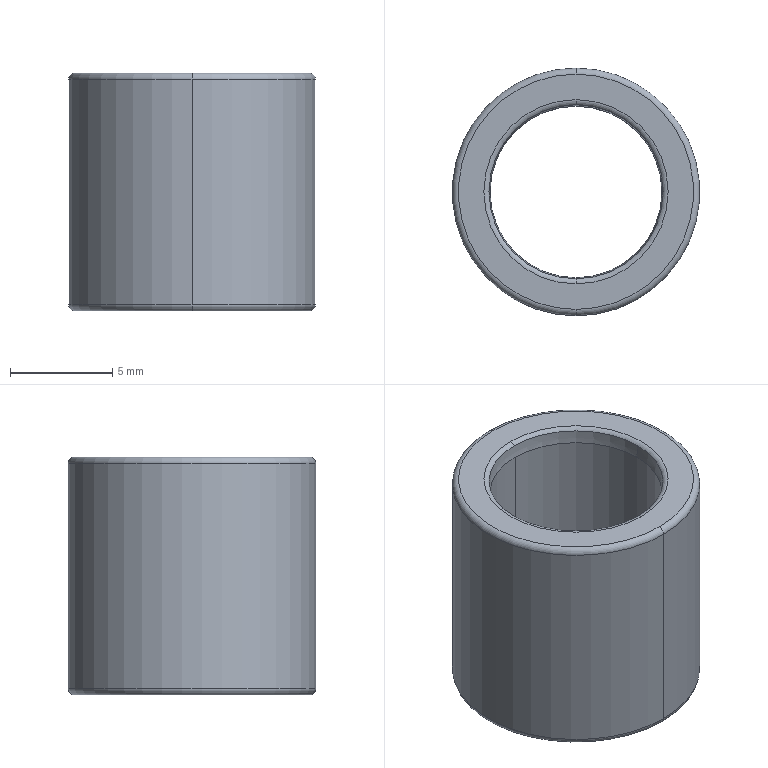Part | STEP file | 12b-1_03 | 1 solid | 16 faces | box 12.07 x 12.07 x 11.6 mm | volume 683.04 mm3 | torus 8 | cylinder 4 | plane 2 | spline 2 | commonest cylinder face diameters 8.39 x2 12.07 x2
STEP:
#1=CARTESIAN_POINT('',(0.,0.,0.));
#2=DIRECTION('',(0.,0.,1.));
#3=DIRECTION('',(1.,0.,0.));
#4=AXIS2_PLACEMENT_3D('',#1,#2,#3);
#5=CARTESIAN_POINT('',(9.525,-4.195,-5.5));
#6=VERTEX_POINT('',#5);
#7=CARTESIAN_POINT('',(9.525,-4.495,-5.8));
#8=VERTEX_POINT('',#7);
#9=CARTESIAN_POINT('',(9.525,-4.495,-5.5));
#10=DIRECTION('',(-1.,0.,0.));
#11=DIRECTION('',(0.,1.,0.));
#12=AXIS2_PLACEMENT_3D('',#9,#10,#11);
#13=CIRCLE('',#12,0.3);
#14=CARTESIAN_POINT('',(9.525,0.,-5.5));
#15=DIRECTION('',(0.,0.,1.));
#16=DIRECTION('',(-0.03665,-0.9993,0.));
#17=AXIS2_PLACEMENT_3D('',#14,#15,#16);
#18=TOROIDAL_SURFACE('',#17,4.495,0.3);
#19=CARTESIAN_POINT('',(0.03666,3.142));
#20=DIRECTION('',(0.,1.));
#21=VECTOR('',#20,1.);
#22=LINE('',#19,#21);
#23=(GEOMETRIC_REPRESENTATION_CONTEXT(2)PARAMETRIC_REPRESENTATION_CONTEXT()REPRESENTATION_CONTEXT('',''));
#24=DEFINITIONAL_REPRESENTATION('',(#22),#23);
#25=PCURVE('',#18,#24);
#26=CARTESIAN_POINT('',(9.525,0.,-5.5));
#27=DIRECTION('',(0.,0.,1.));
#28=DIRECTION('',(0.03665,0.9993,0.));
#29=AXIS2_PLACEMENT_3D('',#26,#27,#28);
#30=TOROIDAL_SURFACE('',#29,4.495,0.3);
#31=CARTESIAN_POINT('',(3.178,3.142));
#32=DIRECTION('',(0.,1.));
#33=VECTOR('',#32,1.);
#34=LINE('',#31,#33);
#35=(GEOMETRIC_REPRESENTATION_CONTEXT(2)PARAMETRIC_REPRESENTATION_CONTEXT()REPRESENTATION_CONTEXT('',''));
#36=DEFINITIONAL_REPRESENTATION('',(#34),#35);
#37=PCURVE('',#30,#36);
#38=SURFACE_CURVE('',#13,(#25,#37),.PCURVE_S1.);
#39=EDGE_CURVE('',#6,#8,#38,.T.);
#40=ORIENTED_EDGE('',*,*,#39,.F.);
#41=CARTESIAN_POINT('',(9.525,4.195,-5.5));
#42=VERTEX_POINT('',#41);
#43=CARTESIAN_POINT('',(9.525,0.,-5.5));
#44=DIRECTION('',(0.,0.,-1.));
#45=DIRECTION('',(0.,1.,0.));
#46=AXIS2_PLACEMENT_3D('',#43,#44,#45);
#47=CIRCLE('',#46,4.195);
#48=CARTESIAN_POINT('',(3.178,3.142));
#49=DIRECTION('',(-1.,0.));
#50=VECTOR('',#49,1.);
#51=LINE('',#48,#50);
#52=(GEOMETRIC_REPRESENTATION_CONTEXT(2)PARAMETRIC_REPRESENTATION_CONTEXT()REPRESENTATION_CONTEXT('',''));
#53=DEFINITIONAL_REPRESENTATION('',(#51),#52);
#54=PCURVE('',#18,#53);
#55=CARTESIAN_POINT('',(9.525,0.,-5.5));
#56=DIRECTION('',(0.,0.,-1.));
#57=DIRECTION('',(0.,1.,0.));
#58=AXIS2_PLACEMENT_3D('',#55,#56,#57);
#59=CYLINDRICAL_SURFACE('',#58,4.195);
#60=CARTESIAN_POINT('',(0.,0.));
#61=DIRECTION('',(1.,0.));
#62=VECTOR('',#61,1.);
#63=LINE('',#60,#62);
#64=(GEOMETRIC_REPRESENTATION_CONTEXT(2)PARAMETRIC_REPRESENTATION_CONTEXT()REPRESENTATION_CONTEXT('',''));
#65=DEFINITIONAL_REPRESENTATION('',(#63),#64);
#66=PCURVE('',#59,#65);
#67=SURFACE_CURVE('',#47,(#54,#66),.PCURVE_S1.);
#68=EDGE_CURVE('',#42,#6,#67,.T.);
#69=ORIENTED_EDGE('',*,*,#68,.F.);
#70=CARTESIAN_POINT('',(9.525,4.495,-5.8));
#71=VERTEX_POINT('',#70);
#72=CARTESIAN_POINT('',(9.525,4.495,-5.5));
#73=DIRECTION('',(-1.,0.,0.));
#74=DIRECTION('',(0.,-0.000000819,-1.));
#75=AXIS2_PLACEMENT_3D('',#72,#73,#74);
#76=CIRCLE('',#75,0.3);
#77=CARTESIAN_POINT('',(3.178,4.712));
#78=DIRECTION('',(0.,-1.));
#79=VECTOR('',#78,1.);
#80=LINE('',#77,#79);
#81=(GEOMETRIC_REPRESENTATION_CONTEXT(2)PARAMETRIC_REPRESENTATION_CONTEXT()REPRESENTATION_CONTEXT('',''));
#82=DEFINITIONAL_REPRESENTATION('',(#80),#81);
#83=PCURVE('',#18,#82);
#84=CARTESIAN_POINT('',(0.03666,4.712));
#85=DIRECTION('',(0.,-1.));
#86=VECTOR('',#85,1.);
#87=LINE('',#84,#86);
#88=(GEOMETRIC_REPRESENTATION_CONTEXT(2)PARAMETRIC_REPRESENTATION_CONTEXT()REPRESENTATION_CONTEXT('',''));
#89=DEFINITIONAL_REPRESENTATION('',(#87),#88);
#90=PCURVE('',#30,#89);
#91=SURFACE_CURVE('',#76,(#83,#90),.PCURVE_S1.);
#92=EDGE_CURVE('',#71,#42,#91,.T.);
#93=ORIENTED_EDGE('',*,*,#92,.F.);
#94=CARTESIAN_POINT('',(9.525,0.,-5.8));
#95=DIRECTION('',(0.,0.,-1.));
#96=DIRECTION('',(0.,1.,0.));
#97=AXIS2_PLACEMENT_3D('',#94,#95,#96);
#98=CIRCLE('',#97,4.495);
#99=CARTESIAN_POINT('',(3.178,4.712));
#100=DIRECTION('',(-1.,0.));
#101=VECTOR('',#100,1.);
#102=LINE('',#99,#101);
#103=(GEOMETRIC_REPRESENTATION_CONTEXT(2)PARAMETRIC_REPRESENTATION_CONTEXT()REPRESENTATION_CONTEXT('',''));
#104=DEFINITIONAL_REPRESENTATION('',(#102),#103);
#105=PCURVE('',#18,#104);
#106=CARTESIAN_POINT('',(9.525,0.,-5.8));
#107=DIRECTION('',(0.,0.,1.));
#108=DIRECTION('',(1.,0.,0.));
#109=AXIS2_PLACEMENT_3D('',#106,#107,#108);
#110=PLANE('',#109);
#111=CARTESIAN_POINT('',(0.,4.495));
#112=CARTESIAN_POINT('',(7.786,4.495));
#113=CARTESIAN_POINT('',(3.893,-2.247));
#114=CARTESIAN_POINT('',(0.,-8.99));
#115=CARTESIAN_POINT('',(-3.893,-2.247));
#116=CARTESIAN_POINT('',(-7.786,4.495));
#117=CARTESIAN_POINT('',(0.,4.495));
#118=(BOUNDED_CURVE()B_SPLINE_CURVE(2,(#111,#112,#113,#114,#115,#116,#117),.UNSPECIFIED.,.T.,.F.)B_SPLINE_CURVE_WITH_KNOTS((1,2,2,2,2,1),(-2.094,0.,2.094,4.189,6.283,8.378),.UNSPECIFIED.)CURVE()GEOMETRIC_REPRESENTATION_ITEM()RATIONAL_B_SPLINE_CURVE((1.,0.5,1.,0.5,1.,0.5,1.))REPRESENTATION_ITEM(''));
#119=(GEOMETRIC_REPRESENTATION_CONTEXT(2)PARAMETRIC_REPRESENTATION_CONTEXT()REPRESENTATION_CONTEXT('',''));
#120=DEFINITIONAL_REPRESENTATION('',(#118),#119);
#121=PCURVE('',#110,#120);
#122=SURFACE_CURVE('',#98,(#105,#121),.PCURVE_S1.);
#123=EDGE_CURVE('',#71,#8,#122,.T.);
#124=ORIENTED_EDGE('',*,*,#123,.T.);
#125=EDGE_LOOP('',(#40,#69,#93,#124));
#126=FACE_BOUND('',#125,.T.);
#127=ADVANCED_FACE('',(#126),#18,.T.);
#128=CARTESIAN_POINT('',(9.525,-5.735,-5.8));
#129=VERTEX_POINT('',#128);
#130=CARTESIAN_POINT('',(9.525,5.735,-5.8));
#131=VERTEX_POINT('',#130);
#132=CARTESIAN_POINT('',(9.525,0.,-5.8));
#133=DIRECTION('',(0.,0.,1.));
#134=DIRECTION('',(0.,-1.,0.));
#135=AXIS2_PLACEMENT_3D('',#132,#133,#134);
#136=CIRCLE('',#135,5.735);
#137=CARTESIAN_POINT('',(0.,0.));
#138=DIRECTION('',(0.,-1.));
#139=AXIS2_PLACEMENT_2D('',#137,#138);
#140=CIRCLE('',#139,5.735);
#141=(GEOMETRIC_REPRESENTATION_CONTEXT(2)PARAMETRIC_REPRESENTATION_CONTEXT()REPRESENTATION_CONTEXT('',''));
#142=DEFINITIONAL_REPRESENTATION('',(#140),#141);
#143=PCURVE('',#110,#142);
#144=CARTESIAN_POINT('',(9.525,0.,-5.5));
#145=DIRECTION('',(0.,0.,1.));
#146=DIRECTION('',(-0.03619,0.9993,0.));
#147=AXIS2_PLACEMENT_3D('',#144,#145,#146);
#148=TOROIDAL_SURFACE('',#147,5.735,0.3);
#149=CARTESIAN_POINT('',(3.105,4.712));
#150=DIRECTION('',(1.,0.));
#151=VECTOR('',#150,1.);
#152=LINE('',#149,#151);
#153=(GEOMETRIC_REPRESENTATION_CONTEXT(2)PARAMETRIC_REPRESENTATION_CONTEXT()REPRESENTATION_CONTEXT('',''));
#154=DEFINITIONAL_REPRESENTATION('',(#152),#153);
#155=PCURVE('',#148,#154);
#156=SURFACE_CURVE('',#136,(#143,#155),.PCURVE_S1.);
#157=EDGE_CURVE('',#129,#131,#156,.T.);
#158=ORIENTED_EDGE('',*,*,#157,.F.);
#159=CARTESIAN_POINT('',(9.525,0.,-5.8));
#160=DIRECTION('',(0.,0.,1.));
#161=DIRECTION('',(0.,1.,0.));
#162=AXIS2_PLACEMENT_3D('',#159,#160,#161);
#163=CIRCLE('',#162,5.735);
#164=CARTESIAN_POINT('',(0.,0.));
#165=DIRECTION('',(0.,1.));
#166=AXIS2_PLACEMENT_2D('',#164,#165);
#167=CIRCLE('',#166,5.735);
#168=(GEOMETRIC_REPRESENTATION_CONTEXT(2)PARAMETRIC_REPRESENTATION_CONTEXT()REPRESENTATION_CONTEXT('',''));
#169=DEFINITIONAL_REPRESENTATION('',(#167),#168);
#170=PCURVE('',#110,#169);
#171=CARTESIAN_POINT('',(9.525,0.,-5.5));
#172=DIRECTION('',(0.,0.,1.));
#173=DIRECTION('',(0.03619,-0.9993,0.));
#174=AXIS2_PLACEMENT_3D('',#171,#172,#173);
#175=TOROIDAL_SURFACE('',#174,5.735,0.3);
#176=CARTESIAN_POINT('',(3.105,4.712));
#177=DIRECTION('',(1.,0.));
#178=VECTOR('',#177,1.);
#179=LINE('',#176,#178);
#180=(GEOMETRIC_REPRESENTATION_CONTEXT(2)PARAMETRIC_REPRESENTATION_CONTEXT()REPRESENTATION_CONTEXT('',''));
#181=DEFINITIONAL_REPRESENTATION('',(#179),#180);
#182=PCURVE('',#175,#181);
#183=SURFACE_CURVE('',#163,(#170,#182),.PCURVE_S1.);
#184=EDGE_CURVE('',#131,#129,#183,.T.);
#185=ORIENTED_EDGE('',*,*,#184,.F.);
#186=EDGE_LOOP('',(#158,#185));
#187=FACE_BOUND('',#186,.T.);
#188=CARTESIAN_POINT('',(9.525,0.,-5.8));
#189=DIRECTION('',(0.,0.,-1.));
#190=DIRECTION('',(0.,-1.,0.));
#191=AXIS2_PLACEMENT_3D('',#188,#189,#190);
#192=CIRCLE('',#191,4.495);
#193=CARTESIAN_POINT('',(0.,-4.495));
#194=CARTESIAN_POINT('',(-7.786,-4.495));
#195=CARTESIAN_POINT('',(-3.893,2.247));
#196=CARTESIAN_POINT('',(0.,8.99));
#197=CARTESIAN_POINT('',(3.893,2.247));
#198=CARTESIAN_POINT('',(7.786,-4.495));
#199=CARTESIAN_POINT('',(0.,-4.495));
#200=(BOUNDED_CURVE()B_SPLINE_CURVE(2,(#193,#194,#195,#196,#197,#198,#199),.UNSPECIFIED.,.T.,.F.)B_SPLINE_CURVE_WITH_KNOTS((1,2,2,2,2,1),(-2.094,0.,2.094,4.189,6.283,8.378),.UNSPECIFIED.)CURVE()GEOMETRIC_REPRESENTATION_ITEM()RATIONAL_B_SPLINE_CURVE((1.,0.5,1.,0.5,1.,0.5,1.))REPRESENTATION_ITEM(''));
#201=(GEOMETRIC_REPRESENTATION_CONTEXT(2)PARAMETRIC_REPRESENTATION_CONTEXT()REPRESENTATION_CONTEXT('',''));
#202=DEFINITIONAL_REPRESENTATION('',(#200),#201);
#203=PCURVE('',#110,#202);
#204=CARTESIAN_POINT('',(3.178,4.712));
#205=DIRECTION('',(-1.,0.));
#206=VECTOR('',#205,1.);
#207=LINE('',#204,#206);
#208=(GEOMETRIC_REPRESENTATION_CONTEXT(2)PARAMETRIC_REPRESENTATION_CONTEXT()REPRESENTATION_CONTEXT('',''));
#209=DEFINITIONAL_REPRESENTATION('',(#207),#208);
#210=PCURVE('',#30,#209);
#211=SURFACE_CURVE('',#192,(#203,#210),.PCURVE_S1.);
#212=EDGE_CURVE('',#8,#71,#211,.T.);
#213=ORIENTED_EDGE('',*,*,#212,.F.);
#214=ORIENTED_EDGE('',*,*,#123,.F.);
#215=EDGE_LOOP('',(#213,#214));
#216=FACE_BOUND('',#215,.T.);
#217=ADVANCED_FACE('',(#187,#216),#110,.F.);
#218=CARTESIAN_POINT('',(9.525,-6.035,-5.5));
#219=VERTEX_POINT('',#218);
#220=CARTESIAN_POINT('',(9.525,-5.735,-5.5));
#221=DIRECTION('',(-1.,0.,0.));
#222=DIRECTION('',(0.,0.000001786,-1.));
#223=AXIS2_PLACEMENT_3D('',#220,#221,#222);
#224=CIRCLE('',#223,0.3);
#225=CARTESIAN_POINT('',(6.247,4.712));
#226=DIRECTION('',(0.,1.));
#227=VECTOR('',#226,1.);
#228=LINE('',#225,#227);
#229=(GEOMETRIC_REPRESENTATION_CONTEXT(2)PARAMETRIC_REPRESENTATION_CONTEXT()REPRESENTATION_CONTEXT('',''));
#230=DEFINITIONAL_REPRESENTATION('',(#228),#229);
#231=PCURVE('',#175,#230);
#232=CARTESIAN_POINT('',(3.105,4.712));
#233=DIRECTION('',(0.,1.));
#234=VECTOR('',#233,1.);
#235=LINE('',#232,#234);
#236=(GEOMETRIC_REPRESENTATION_CONTEXT(2)PARAMETRIC_REPRESENTATION_CONTEXT()REPRESENTATION_CONTEXT('',''));
#237=DEFINITIONAL_REPRESENTATION('',(#235),#236);
#238=PCURVE('',#148,#237);
#239=SURFACE_CURVE('',#224,(#231,#238),.PCURVE_S1.);
#240=EDGE_CURVE('',#129,#219,#239,.T.);
#241=ORIENTED_EDGE('',*,*,#240,.T.);
#242=CARTESIAN_POINT('',(9.525,6.035,-5.5));
#243=VERTEX_POINT('',#242);
#244=CARTESIAN_POINT('',(9.525,0.,-5.5));
#245=DIRECTION('',(0.,0.,-1.));
#246=DIRECTION('',(0.000000001,-1.,0.));
#247=AXIS2_PLACEMENT_3D('',#244,#245,#246);
#248=CIRCLE('',#247,6.035);
#249=CARTESIAN_POINT('',(6.247,6.283));
#250=DIRECTION('',(-1.,0.));
#251=VECTOR('',#250,1.);
#252=LINE('',#249,#251);
#253=(GEOMETRIC_REPRESENTATION_CONTEXT(2)PARAMETRIC_REPRESENTATION_CONTEXT()REPRESENTATION_CONTEXT('',''));
#254=DEFINITIONAL_REPRESENTATION('',(#252),#253);
#255=PCURVE('',#175,#254);
#256=CARTESIAN_POINT('',(9.525,0.,-5.5));
#257=DIRECTION('',(0.,0.,-1.));
#258=DIRECTION('',(0.,1.,0.));
#259=AXIS2_PLACEMENT_3D('',#256,#257,#258);
#260=CYLINDRICAL_SURFACE('',#259,6.035);
#261=CARTESIAN_POINT('',(3.142,0.));
#262=DIRECTION('',(1.,0.));
#263=VECTOR('',#262,1.);
#264=LINE('',#261,#263);
#265=(GEOMETRIC_REPRESENTATION_CONTEXT(2)PARAMETRIC_REPRESENTATION_CONTEXT()REPRESENTATION_CONTEXT('',''));
#266=DEFINITIONAL_REPRESENTATION('',(#264),#265);
#267=PCURVE('',#260,#266);
#268=SURFACE_CURVE('',#248,(#255,#267),.PCURVE_S1.);
#269=EDGE_CURVE('',#219,#243,#268,.T.);
#270=ORIENTED_EDGE('',*,*,#269,.T.);
#271=CARTESIAN_POINT('',(9.525,5.735,-5.5));
#272=DIRECTION('',(-1.,0.,0.));
#273=DIRECTION('',(0.,1.,0.));
#274=AXIS2_PLACEMENT_3D('',#271,#272,#273);
#275=CIRCLE('',#274,0.3);
#276=CARTESIAN_POINT('',(3.105,6.283));
#277=DIRECTION('',(0.,-1.));
#278=VECTOR('',#277,1.);
#279=LINE('',#276,#278);
#280=(GEOMETRIC_REPRESENTATION_CONTEXT(2)PARAMETRIC_REPRESENTATION_CONTEXT()REPRESENTATION_CONTEXT('',''));
#281=DEFINITIONAL_REPRESENTATION('',(#279),#280);
#282=PCURVE('',#175,#281);
#283=CARTESIAN_POINT('',(6.247,6.283));
#284=DIRECTION('',(0.,-1.));
#285=VECTOR('',#284,1.);
#286=LINE('',#283,#285);
#287=(GEOMETRIC_REPRESENTATION_CONTEXT(2)PARAMETRIC_REPRESENTATION_CONTEXT()REPRESENTATION_CONTEXT('',''));
#288=DEFINITIONAL_REPRESENTATION('',(#286),#287);
#289=PCURVE('',#148,#288);
#290=SURFACE_CURVE('',#275,(#282,#289),.PCURVE_S1.);
#291=EDGE_CURVE('',#243,#131,#290,.T.);
#292=ORIENTED_EDGE('',*,*,#291,.T.);
#293=ORIENTED_EDGE('',*,*,#184,.T.);
#294=EDGE_LOOP('',(#241,#270,#292,#293));
#295=FACE_BOUND('',#294,.T.);
#296=ADVANCED_FACE('',(#295),#175,.T.);
#297=ORIENTED_EDGE('',*,*,#291,.F.);
#298=CARTESIAN_POINT('',(9.525,0.,-5.5));
#299=DIRECTION('',(0.,0.,-1.));
#300=DIRECTION('',(0.,1.,0.));
#301=AXIS2_PLACEMENT_3D('',#298,#299,#300);
#302=CIRCLE('',#301,6.035);
#303=CARTESIAN_POINT('',(6.247,6.283));
#304=DIRECTION('',(-1.,0.));
#305=VECTOR('',#304,1.);
#306=LINE('',#303,#305);
#307=(GEOMETRIC_REPRESENTATION_CONTEXT(2)PARAMETRIC_REPRESENTATION_CONTEXT()REPRESENTATION_CONTEXT('',''));
#308=DEFINITIONAL_REPRESENTATION('',(#306),#307);
#309=PCURVE('',#148,#308);
#310=CARTESIAN_POINT('',(9.525,0.,-5.5));
#311=DIRECTION('',(0.,0.,-1.));
#312=DIRECTION('',(0.,1.,0.));
#313=AXIS2_PLACEMENT_3D('',#310,#311,#312);
#314=CYLINDRICAL_SURFACE('',#313,6.035);
#315=CARTESIAN_POINT('',(0.,0.));
#316=DIRECTION('',(1.,0.));
#317=VECTOR('',#316,1.);
#318=LINE('',#315,#317);
#319=(GEOMETRIC_REPRESENTATION_CONTEXT(2)PARAMETRIC_REPRESENTATION_CONTEXT()REPRESENTATION_CONTEXT('',''));
#320=DEFINITIONAL_REPRESENTATION('',(#318),#319);
#321=PCURVE('',#314,#320);
#322=SURFACE_CURVE('',#302,(#309,#321),.PCURVE_S1.);
#323=EDGE_CURVE('',#243,#219,#322,.T.);
#324=ORIENTED_EDGE('',*,*,#323,.T.);
#325=ORIENTED_EDGE('',*,*,#240,.F.);
#326=ORIENTED_EDGE('',*,*,#157,.T.);
#327=EDGE_LOOP('',(#297,#324,#325,#326));
#328=FACE_BOUND('',#327,.T.);
#329=ADVANCED_FACE('',(#328),#148,.T.);
#330=CARTESIAN_POINT('',(9.525,-6.035,5.5));
#331=VERTEX_POINT('',#330);
#332=CARTESIAN_POINT('',(9.525,-6.035,5.5));
#333=DIRECTION('',(0.,0.,-1.));
#334=VECTOR('',#333,1.);
#335=LINE('',#332,#334);
#336=CARTESIAN_POINT('',(3.142,-11.));
#337=DIRECTION('',(0.,1.));
#338=VECTOR('',#337,1.);
#339=LINE('',#336,#338);
#340=(GEOMETRIC_REPRESENTATION_CONTEXT(2)PARAMETRIC_REPRESENTATION_CONTEXT()REPRESENTATION_CONTEXT('',''));
#341=DEFINITIONAL_REPRESENTATION('',(#339),#340);
#342=PCURVE('',#314,#341);
#343=CARTESIAN_POINT('',(3.142,-11.));
#344=DIRECTION('',(0.,1.));
#345=VECTOR('',#344,1.);
#346=LINE('',#343,#345);
#347=(GEOMETRIC_REPRESENTATION_CONTEXT(2)PARAMETRIC_REPRESENTATION_CONTEXT()REPRESENTATION_CONTEXT('',''));
#348=DEFINITIONAL_REPRESENTATION('',(#346),#347);
#349=PCURVE('',#260,#348);
#350=SURFACE_CURVE('',#335,(#342,#349),.PCURVE_S1.);
#351=EDGE_CURVE('',#331,#219,#350,.T.);
#352=ORIENTED_EDGE('',*,*,#351,.T.);
#353=ORIENTED_EDGE('',*,*,#323,.F.);
#354=CARTESIAN_POINT('',(9.525,6.035,5.5));
#355=VERTEX_POINT('',#354);
#356=CARTESIAN_POINT('',(9.525,6.035,-5.5));
#357=DIRECTION('',(0.,0.,1.));
#358=VECTOR('',#357,1.);
#359=LINE('',#356,#358);
#360=CARTESIAN_POINT('',(0.,0.));
#361=DIRECTION('',(0.,-1.));
#362=VECTOR('',#361,1.);
#363=LINE('',#360,#362);
#364=(GEOMETRIC_REPRESENTATION_CONTEXT(2)PARAMETRIC_REPRESENTATION_CONTEXT()REPRESENTATION_CONTEXT('',''));
#365=DEFINITIONAL_REPRESENTATION('',(#363),#364);
#366=PCURVE('',#314,#365);
#367=CARTESIAN_POINT('',(6.283,0.));
#368=DIRECTION('',(0.,-1.));
#369=VECTOR('',#368,1.);
#370=LINE('',#367,#369);
#371=(GEOMETRIC_REPRESENTATION_CONTEXT(2)PARAMETRIC_REPRESENTATION_CONTEXT()REPRESENTATION_CONTEXT('',''));
#372=DEFINITIONAL_REPRESENTATION('',(#370),#371);
#373=PCURVE('',#260,#372);
#374=SURFACE_CURVE('',#359,(#366,#373),.PCURVE_S1.);
#375=EDGE_CURVE('',#243,#355,#374,.T.);
#376=ORIENTED_EDGE('',*,*,#375,.T.);
#377=CARTESIAN_POINT('',(9.525,0.,5.5));
#378=DIRECTION('',(0.,0.,-1.));
#379=DIRECTION('',(0.,1.,0.));
#380=AXIS2_PLACEMENT_3D('',#377,#378,#379);
#381=CIRCLE('',#380,6.035);
#382=CARTESIAN_POINT('',(0.,-11.));
#383=DIRECTION('',(1.,0.));
#384=VECTOR('',#383,1.);
#385=LINE('',#382,#384);
#386=(GEOMETRIC_REPRESENTATION_CONTEXT(2)PARAMETRIC_REPRESENTATION_CONTEXT()REPRESENTATION_CONTEXT('',''));
#387=DEFINITIONAL_REPRESENTATION('',(#385),#386);
#388=PCURVE('',#314,#387);
#389=CARTESIAN_POINT('',(9.525,0.,5.5));
#390=DIRECTION('',(0.,0.,1.));
#391=DIRECTION('',(-0.02548,-0.9997,0.));
#392=AXIS2_PLACEMENT_3D('',#389,#390,#391);
#393=TOROIDAL_SURFACE('',#392,5.735,0.3);
#394=CARTESIAN_POINT('',(3.167,0.));
#395=DIRECTION('',(-1.,0.));
#396=VECTOR('',#395,1.);
#397=LINE('',#394,#396);
#398=(GEOMETRIC_REPRESENTATION_CONTEXT(2)PARAMETRIC_REPRESENTATION_CONTEXT()REPRESENTATION_CONTEXT('',''));
#399=DEFINITIONAL_REPRESENTATION('',(#397),#398);
#400=PCURVE('',#393,#399);
#401=SURFACE_CURVE('',#381,(#388,#400),.PCURVE_S1.);
#402=EDGE_CURVE('',#355,#331,#401,.T.);
#403=ORIENTED_EDGE('',*,*,#402,.T.);
#404=EDGE_LOOP('',(#352,#353,#376,#403));
#405=FACE_BOUND('',#404,.T.);
#406=ADVANCED_FACE('',(#405),#314,.T.);
#407=CARTESIAN_POINT('',(9.525,-5.735,5.8));
#408=VERTEX_POINT('',#407);
#409=CARTESIAN_POINT('',(9.525,-5.735,5.5));
#410=DIRECTION('',(1.,0.,0.));
#411=DIRECTION('',(0.,0.000001986,1.));
#412=AXIS2_PLACEMENT_3D('',#409,#410,#411);
#413=CIRCLE('',#412,0.3);
#414=CARTESIAN_POINT('',(0.02548,1.571));
#415=DIRECTION('',(0.,-1.));
#416=VECTOR('',#415,1.);
#417=LINE('',#414,#416);
#418=(GEOMETRIC_REPRESENTATION_CONTEXT(2)PARAMETRIC_REPRESENTATION_CONTEXT()REPRESENTATION_CONTEXT('',''));
#419=DEFINITIONAL_REPRESENTATION('',(#417),#418);
#420=PCURVE('',#393,#419);
#421=CARTESIAN_POINT('',(9.525,0.,5.5));
#422=DIRECTION('',(0.,0.,1.));
#423=DIRECTION('',(0.02548,0.9997,0.));
#424=AXIS2_PLACEMENT_3D('',#421,#422,#423);
#425=TOROIDAL_SURFACE('',#424,5.735,0.3);
#426=CARTESIAN_POINT('',(3.167,1.571));
#427=DIRECTION('',(0.,-1.));
#428=VECTOR('',#427,1.);
#429=LINE('',#426,#428);
#430=(GEOMETRIC_REPRESENTATION_CONTEXT(2)PARAMETRIC_REPRESENTATION_CONTEXT()REPRESENTATION_CONTEXT('',''));
#431=DEFINITIONAL_REPRESENTATION('',(#429),#430);
#432=PCURVE('',#425,#431);
#433=SURFACE_CURVE('',#413,(#420,#432),.PCURVE_S1.);
#434=EDGE_CURVE('',#408,#331,#433,.T.);
#435=ORIENTED_EDGE('',*,*,#434,.T.);
#436=ORIENTED_EDGE('',*,*,#402,.F.);
#437=CARTESIAN_POINT('',(9.525,5.735,5.8));
#438=VERTEX_POINT('',#437);
#439=CARTESIAN_POINT('',(9.525,5.735,5.5));
#440=DIRECTION('',(1.,0.,0.));
#441=DIRECTION('',(0.,1.,0.));
#442=AXIS2_PLACEMENT_3D('',#439,#440,#441);
#443=CIRCLE('',#442,0.3);
#444=CARTESIAN_POINT('',(3.167,0.));
#445=DIRECTION('',(0.,1.));
#446=VECTOR('',#445,1.);
#447=LINE('',#444,#446);
#448=(GEOMETRIC_REPRESENTATION_CONTEXT(2)PARAMETRIC_REPRESENTATION_CONTEXT()REPRESENTATION_CONTEXT('',''));
#449=DEFINITIONAL_REPRESENTATION('',(#447),#448);
#450=PCURVE('',#393,#449);
#451=CARTESIAN_POINT('',(0.02548,0.));
#452=DIRECTION('',(0.,1.));
#453=VECTOR('',#452,1.);
#454=LINE('',#451,#453);
#455=(GEOMETRIC_REPRESENTATION_CONTEXT(2)PARAMETRIC_REPRESENTATION_CONTEXT()REPRESENTATION_CONTEXT('',''));
#456=DEFINITIONAL_REPRESENTATION('',(#454),#455);
#457=PCURVE('',#425,#456);
#458=SURFACE_CURVE('',#443,(#450,#457),.PCURVE_S1.);
#459=EDGE_CURVE('',#355,#438,#458,.T.);
#460=ORIENTED_EDGE('',*,*,#459,.T.);
#461=CARTESIAN_POINT('',(9.525,0.,5.8));
#462=DIRECTION('',(0.,0.,-1.));
#463=DIRECTION('',(0.,1.,0.));
#464=AXIS2_PLACEMENT_3D('',#461,#462,#463);
#465=CIRCLE('',#464,5.735);
#466=CARTESIAN_POINT('',(3.167,1.571));
#467=DIRECTION('',(-1.,0.));
#468=VECTOR('',#467,1.);
#469=LINE('',#466,#468);
#470=(GEOMETRIC_REPRESENTATION_CONTEXT(2)PARAMETRIC_REPRESENTATION_CONTEXT()REPRESENTATION_CONTEXT('',''));
#471=DEFINITIONAL_REPRESENTATION('',(#469),#470);
#472=PCURVE('',#393,#471);
#473=CARTESIAN_POINT('',(9.525,0.,5.8));
#474=DIRECTION('',(0.,0.,1.));
#475=DIRECTION('',(1.,0.,0.));
#476=AXIS2_PLACEMENT_3D('',#473,#474,#475);
#477=PLANE('',#476);
#478=CARTESIAN_POINT('',(0.,5.735));
#479=CARTESIAN_POINT('',(9.933,5.735));
#480=CARTESIAN_POINT('',(4.967,-2.867));
#481=CARTESIAN_POINT('',(0.,-11.47));
#482=CARTESIAN_POINT('',(-4.967,-2.867));
#483=CARTESIAN_POINT('',(-9.933,5.735));
#484=CARTESIAN_POINT('',(0.,5.735));
#485=(BOUNDED_CURVE()B_SPLINE_CURVE(2,(#478,#479,#480,#481,#482,#483,#484),.UNSPECIFIED.,.T.,.F.)B_SPLINE_CURVE_WITH_KNOTS((1,2,2,2,2,1),(-2.094,0.,2.094,4.189,6.283,8.378),.UNSPECIFIED.)CURVE()GEOMETRIC_REPRESENTATION_ITEM()RATIONAL_B_SPLINE_CURVE((1.,0.5,1.,0.5,1.,0.5,1.))REPRESENTATION_ITEM(''));
#486=(GEOMETRIC_REPRESENTATION_CONTEXT(2)PARAMETRIC_REPRESENTATION_CONTEXT()REPRESENTATION_CONTEXT('',''));
#487=DEFINITIONAL_REPRESENTATION('',(#485),#486);
#488=PCURVE('',#477,#487);
#489=SURFACE_CURVE('',#465,(#472,#488),.PCURVE_S1.);
#490=EDGE_CURVE('',#438,#408,#489,.T.);
#491=ORIENTED_EDGE('',*,*,#490,.T.);
#492=EDGE_LOOP('',(#435,#436,#460,#491));
#493=FACE_BOUND('',#492,.T.);
#494=ADVANCED_FACE('',(#493),#393,.T.);
#495=ORIENTED_EDGE('',*,*,#490,.F.);
#496=CARTESIAN_POINT('',(9.525,0.,5.8));
#497=DIRECTION('',(0.,0.,-1.));
#498=DIRECTION('',(0.,-1.,0.));
#499=AXIS2_PLACEMENT_3D('',#496,#497,#498);
#500=CIRCLE('',#499,5.735);
#501=CARTESIAN_POINT('',(0.,-5.735));
#502=CARTESIAN_POINT('',(-9.933,-5.735));
#503=CARTESIAN_POINT('',(-4.967,2.867));
#504=CARTESIAN_POINT('',(0.,11.47));
#505=CARTESIAN_POINT('',(4.967,2.867));
#506=CARTESIAN_POINT('',(9.933,-5.735));
#507=CARTESIAN_POINT('',(0.,-5.735));
#508=(BOUNDED_CURVE()B_SPLINE_CURVE(2,(#501,#502,#503,#504,#505,#506,#507),.UNSPECIFIED.,.T.,.F.)B_SPLINE_CURVE_WITH_KNOTS((1,2,2,2,2,1),(-2.094,0.,2.094,4.189,6.283,8.378),.UNSPECIFIED.)CURVE()GEOMETRIC_REPRESENTATION_ITEM()RATIONAL_B_SPLINE_CURVE((1.,0.5,1.,0.5,1.,0.5,1.))REPRESENTATION_ITEM(''));
#509=(GEOMETRIC_REPRESENTATION_CONTEXT(2)PARAMETRIC_REPRESENTATION_CONTEXT()REPRESENTATION_CONTEXT('',''));
#510=DEFINITIONAL_REPRESENTATION('',(#508),#509);
#511=PCURVE('',#477,#510);
#512=CARTESIAN_POINT('',(3.167,1.571));
#513=DIRECTION('',(-1.,0.));
#514=VECTOR('',#513,1.);
#515=LINE('',#512,#514);
#516=(GEOMETRIC_REPRESENTATION_CONTEXT(2)PARAMETRIC_REPRESENTATION_CONTEXT()REPRESENTATION_CONTEXT('',''));
#517=DEFINITIONAL_REPRESENTATION('',(#515),#516);
#518=PCURVE('',#425,#517);
#519=SURFACE_CURVE('',#500,(#511,#518),.PCURVE_S1.);
#520=EDGE_CURVE('',#408,#438,#519,.T.);
#521=ORIENTED_EDGE('',*,*,#520,.F.);
#522=EDGE_LOOP('',(#495,#521));
#523=FACE_BOUND('',#522,.T.);
#524=CARTESIAN_POINT('',(9.525,4.495,5.8));
#525=VERTEX_POINT('',#524);
#526=CARTESIAN_POINT('',(9.525,-4.495,5.8));
#527=VERTEX_POINT('',#526);
#528=CARTESIAN_POINT('',(9.525,0.,5.8));
#529=DIRECTION('',(0.,0.,1.));
#530=DIRECTION('',(0.,1.,0.));
#531=AXIS2_PLACEMENT_3D('',#528,#529,#530);
#532=CIRCLE('',#531,4.495);
#533=CARTESIAN_POINT('',(0.,0.));
#534=DIRECTION('',(0.,1.));
#535=AXIS2_PLACEMENT_2D('',#533,#534);
#536=CIRCLE('',#535,4.495);
#537=(GEOMETRIC_REPRESENTATION_CONTEXT(2)PARAMETRIC_REPRESENTATION_CONTEXT()REPRESENTATION_CONTEXT('',''));
#538=DEFINITIONAL_REPRESENTATION('',(#536),#537);
#539=PCURVE('',#477,#538);
#540=CARTESIAN_POINT('',(9.525,0.,5.5));
#541=DIRECTION('',(0.,0.,1.));
#542=DIRECTION('',(0.05205,-0.9986,0.));
#543=AXIS2_PLACEMENT_3D('',#540,#541,#542);
#544=TOROIDAL_SURFACE('',#543,4.495,0.3);
#545=CARTESIAN_POINT('',(3.09,1.571));
#546=DIRECTION('',(1.,0.));
#547=VECTOR('',#546,1.);
#548=LINE('',#545,#547);
#549=(GEOMETRIC_REPRESENTATION_CONTEXT(2)PARAMETRIC_REPRESENTATION_CONTEXT()REPRESENTATION_CONTEXT('',''));
#550=DEFINITIONAL_REPRESENTATION('',(#548),#549);
#551=PCURVE('',#544,#550);
#552=SURFACE_CURVE('',#532,(#539,#551),.PCURVE_S1.);
#553=EDGE_CURVE('',#525,#527,#552,.T.);
#554=ORIENTED_EDGE('',*,*,#553,.F.);
#555=CARTESIAN_POINT('',(9.525,0.,5.8));
#556=DIRECTION('',(0.,0.,1.));
#557=DIRECTION('',(0.,-1.,0.));
#558=AXIS2_PLACEMENT_3D('',#555,#556,#557);
#559=CIRCLE('',#558,4.495);
#560=CARTESIAN_POINT('',(0.,0.));
#561=DIRECTION('',(0.,-1.));
#562=AXIS2_PLACEMENT_2D('',#560,#561);
#563=CIRCLE('',#562,4.495);
#564=(GEOMETRIC_REPRESENTATION_CONTEXT(2)PARAMETRIC_REPRESENTATION_CONTEXT()REPRESENTATION_CONTEXT('',''));
#565=DEFINITIONAL_REPRESENTATION('',(#563),#564);
#566=PCURVE('',#477,#565);
#567=CARTESIAN_POINT('',(9.525,0.,5.5));
#568=DIRECTION('',(0.,0.,1.));
#569=DIRECTION('',(-0.05205,0.9986,0.));
#570=AXIS2_PLACEMENT_3D('',#567,#568,#569);
#571=TOROIDAL_SURFACE('',#570,4.495,0.3);
#572=CARTESIAN_POINT('',(3.09,1.571));
#573=DIRECTION('',(1.,0.));
#574=VECTOR('',#573,1.);
#575=LINE('',#572,#574);
#576=(GEOMETRIC_REPRESENTATION_CONTEXT(2)PARAMETRIC_REPRESENTATION_CONTEXT()REPRESENTATION_CONTEXT('',''));
#577=DEFINITIONAL_REPRESENTATION('',(#575),#576);
#578=PCURVE('',#571,#577);
#579=SURFACE_CURVE('',#559,(#566,#578),.PCURVE_S1.);
#580=EDGE_CURVE('',#527,#525,#579,.T.);
#581=ORIENTED_EDGE('',*,*,#580,.F.);
#582=EDGE_LOOP('',(#554,#581));
#583=FACE_BOUND('',#582,.T.);
#584=ADVANCED_FACE('',(#523,#583),#477,.T.);
#585=ORIENTED_EDGE('',*,*,#459,.F.);
#586=CARTESIAN_POINT('',(9.525,0.,5.5));
#587=DIRECTION('',(0.,0.,1.));
#588=DIRECTION('',(0.,1.,0.));
#589=AXIS2_PLACEMENT_3D('',#586,#587,#588);
#590=CIRCLE('',#589,6.035);
#591=CARTESIAN_POINT('',(0.02548,0.));
#592=DIRECTION('',(1.,0.));
#593=VECTOR('',#592,1.);
#594=LINE('',#591,#593);
#595=(GEOMETRIC_REPRESENTATION_CONTEXT(2)PARAMETRIC_REPRESENTATION_CONTEXT()REPRESENTATION_CONTEXT('',''));
#596=DEFINITIONAL_REPRESENTATION('',(#594),#595);
#597=PCURVE('',#425,#596);
#598=CARTESIAN_POINT('',(6.283,-11.));
#599=DIRECTION('',(-1.,0.));
#600=VECTOR('',#599,1.);
#601=LINE('',#598,#600);
#602=(GEOMETRIC_REPRESENTATION_CONTEXT(2)PARAMETRIC_REPRESENTATION_CONTEXT()REPRESENTATION_CONTEXT('',''));
#603=DEFINITIONAL_REPRESENTATION('',(#601),#602);
#604=PCURVE('',#260,#603);
#605=SURFACE_CURVE('',#590,(#597,#604),.PCURVE_S1.);
#606=EDGE_CURVE('',#355,#331,#605,.T.);
#607=ORIENTED_EDGE('',*,*,#606,.T.);
#608=ORIENTED_EDGE('',*,*,#434,.F.);
#609=ORIENTED_EDGE('',*,*,#520,.T.);
#610=EDGE_LOOP('',(#585,#607,#608,#609));
#611=FACE_BOUND('',#610,.T.);
#612=ADVANCED_FACE('',(#611),#425,.T.);
#613=ORIENTED_EDGE('',*,*,#375,.F.);
#614=ORIENTED_EDGE('',*,*,#269,.F.);
#615=ORIENTED_EDGE('',*,*,#351,.F.);
#616=ORIENTED_EDGE('',*,*,#606,.F.);
#617=EDGE_LOOP('',(#613,#614,#615,#616));
#618=FACE_BOUND('',#617,.T.);
#619=ADVANCED_FACE('',(#618),#260,.T.);
#620=CARTESIAN_POINT('',(13.77,0.,5.666));
#621=VERTEX_POINT('',#620);
#622=CARTESIAN_POINT('',(9.525,-4.245,5.666));
#623=VERTEX_POINT('',#622);
#624=CARTESIAN_POINT('',(9.525,0.,5.666));
#625=DIRECTION('',(0.,0.,-1.));
#626=DIRECTION('',(1.,0.,0.));
#627=AXIS2_PLACEMENT_3D('',#624,#625,#626);
#628=CIRCLE('',#627,4.245);
#629=CARTESIAN_POINT('',(4.66,2.556));
#630=DIRECTION('',(-1.,0.));
#631=VECTOR('',#630,1.);
#632=LINE('',#629,#631);
#633=(GEOMETRIC_REPRESENTATION_CONTEXT(2)PARAMETRIC_REPRESENTATION_CONTEXT()REPRESENTATION_CONTEXT('',''));
#634=DEFINITIONAL_REPRESENTATION('',(#632),#633);
#635=PCURVE('',#571,#634);
#636=CARTESIAN_POINT('',(5.28,0.,5.666));
#637=CARTESIAN_POINT('',(5.28,-4.245,5.666));
#638=CARTESIAN_POINT('',(9.525,-4.245,5.666));
#639=CARTESIAN_POINT('',(13.77,-4.245,5.666));
#640=CARTESIAN_POINT('',(13.77,0.,5.666));
#641=CARTESIAN_POINT('',(5.284,0.,5.636));
#642=CARTESIAN_POINT('',(5.284,-4.241,5.636));
#643=CARTESIAN_POINT('',(9.525,-4.241,5.636));
#644=CARTESIAN_POINT('',(13.766,-4.241,5.636));
#645=CARTESIAN_POINT('',(13.766,0.,5.636));
#646=CARTESIAN_POINT('',(5.297,0.,5.5));
#647=CARTESIAN_POINT('',(5.297,-4.228,5.5));
#648=CARTESIAN_POINT('',(9.525,-4.228,5.5));
#649=CARTESIAN_POINT('',(13.753,-4.228,5.5));
#650=CARTESIAN_POINT('',(13.753,0.,5.5));
#651=CARTESIAN_POINT('',(5.297,0.,5.277));
#652=CARTESIAN_POINT('',(5.297,-4.228,5.277));
#653=CARTESIAN_POINT('',(9.525,-4.228,5.277));
#654=CARTESIAN_POINT('',(13.753,-4.228,5.277));
#655=CARTESIAN_POINT('',(13.753,0.,5.277));
#656=CARTESIAN_POINT('',(5.313,0.,5.085));
#657=CARTESIAN_POINT('',(5.313,-4.212,5.085));
#658=CARTESIAN_POINT('',(9.525,-4.212,5.085));
#659=CARTESIAN_POINT('',(13.737,-4.212,5.085));
#660=CARTESIAN_POINT('',(13.737,0.,5.085));
#661=CARTESIAN_POINT('',(5.33,0.,5.));
#662=CARTESIAN_POINT('',(5.33,-4.195,5.));
#663=CARTESIAN_POINT('',(9.525,-4.195,5.));
#664=CARTESIAN_POINT('',(13.72,-4.195,5.));
#665=CARTESIAN_POINT('',(13.72,0.,5.));
#666=(BOUNDED_SURFACE()B_SPLINE_SURFACE(3,2,((#636,#637,#638,#639,#640),(#641,#642,#643,#644,#645),(#646,#647,#648,#649,#650),(#651,#652,#653,#654,#655),(#656,#657,#658,#659,#660),(#661,#662,#663,#664,#665)),.UNSPECIFIED.,.F.,.F.,.F.)B_SPLINE_SURFACE_WITH_KNOTS((4,1,1,4),(3,2,3),(0.,0.1351,0.6114,1.),(0.,1.571,3.142),.UNSPECIFIED.)GEOMETRIC_REPRESENTATION_ITEM()RATIONAL_B_SPLINE_SURFACE(((1.,0.7071,1.,0.7071,1.),(1.,0.7071,1.,0.7071,1.),(1.,0.7071,1.,0.7071,1.),(1.,0.7071,1.,0.7071,1.),(1.,0.7071,1.,0.7071,1.),(1.,0.7071,1.,0.7071,1.)))REPRESENTATION_ITEM('')SURFACE());
#667=CARTESIAN_POINT('',(0.,3.142));
#668=CARTESIAN_POINT('',(0.,3.115));
#669=CARTESIAN_POINT('',(0.,3.063));
#670=CARTESIAN_POINT('',(0.,2.987));
#671=CARTESIAN_POINT('',(0.,2.913));
#672=CARTESIAN_POINT('',(0.,2.84));
#673=CARTESIAN_POINT('',(0.,2.768));
#674=CARTESIAN_POINT('',(0.,2.698));
#675=CARTESIAN_POINT('',(0.,2.629));
#676=CARTESIAN_POINT('',(0.,2.56));
#677=CARTESIAN_POINT('',(0.,2.492));
#678=CARTESIAN_POINT('',(0.,2.424));
#679=CARTESIAN_POINT('',(0.,2.356));
#680=CARTESIAN_POINT('',(0.,2.289));
#681=CARTESIAN_POINT('',(0.,2.221));
#682=CARTESIAN_POINT('',(0.,2.152));
#683=CARTESIAN_POINT('',(0.,2.084));
#684=CARTESIAN_POINT('',(0.,2.014));
#685=CARTESIAN_POINT('',(0.,1.944));
#686=CARTESIAN_POINT('',(0.,1.872));
#687=CARTESIAN_POINT('',(0.,1.8));
#688=CARTESIAN_POINT('',(0.,1.725));
#689=CARTESIAN_POINT('',(0.,1.649));
#690=CARTESIAN_POINT('',(0.,1.597));
#691=CARTESIAN_POINT('',(0.,1.571));
#692=B_SPLINE_CURVE_WITH_KNOTS('',3,(#667,#668,#669,#670,#671,#672,#673,#674,#675,#676,#677,#678,#679,#680,#681,#682,#683,#684,#685,#686,#687,#688,#689,#690,#691),.UNSPECIFIED.,.F.,.F.,(4,1,1,1,1,1,1,1,1,1,1,1,1,1,1,1,1,1,1,1,1,1,4),(0.,0.0714,0.1428,0.2142,0.2856,0.357,0.4284,0.4998,0.5712,0.6426,0.714,0.7854,0.8568,0.9282,0.9996,1.071,1.142,1.214,1.285,1.357,1.428,1.499,1.571),.QUASI_UNIFORM_KNOTS.);
#693=(GEOMETRIC_REPRESENTATION_CONTEXT(2)PARAMETRIC_REPRESENTATION_CONTEXT()REPRESENTATION_CONTEXT('',''));
#694=DEFINITIONAL_REPRESENTATION('',(#692),#693);
#695=PCURVE('',#666,#694);
#696=SURFACE_CURVE('',#628,(#635,#695),.PCURVE_S1.);
#697=EDGE_CURVE('',#621,#623,#696,.T.);
#698=ORIENTED_EDGE('',*,*,#697,.T.);
#699=CARTESIAN_POINT('',(9.525,-4.495,5.5));
#700=DIRECTION('',(1.,0.,0.));
#701=DIRECTION('',(0.,0.8333,0.5528));
#702=AXIS2_PLACEMENT_3D('',#699,#700,#701);
#703=CIRCLE('',#702,0.3);
#704=CARTESIAN_POINT('',(3.09,2.556));
#705=DIRECTION('',(0.,-1.));
#706=VECTOR('',#705,1.);
#707=LINE('',#704,#706);
#708=(GEOMETRIC_REPRESENTATION_CONTEXT(2)PARAMETRIC_REPRESENTATION_CONTEXT()REPRESENTATION_CONTEXT('',''));
#709=DEFINITIONAL_REPRESENTATION('',(#707),#708);
#710=PCURVE('',#571,#709);
#711=CARTESIAN_POINT('',(6.231,2.556));
#712=DIRECTION('',(0.,-1.));
#713=VECTOR('',#712,1.);
#714=LINE('',#711,#713);
#715=(GEOMETRIC_REPRESENTATION_CONTEXT(2)PARAMETRIC_REPRESENTATION_CONTEXT()REPRESENTATION_CONTEXT('',''));
#716=DEFINITIONAL_REPRESENTATION('',(#714),#715);
#717=PCURVE('',#544,#716);
#718=SURFACE_CURVE('',#703,(#710,#717),.PCURVE_S1.);
#719=EDGE_CURVE('',#623,#527,#718,.T.);
#720=ORIENTED_EDGE('',*,*,#719,.T.);
#721=ORIENTED_EDGE('',*,*,#580,.T.);
#722=CARTESIAN_POINT('',(9.525,4.245,5.666));
#723=VERTEX_POINT('',#722);
#724=CARTESIAN_POINT('',(9.525,4.495,5.5));
#725=DIRECTION('',(1.,0.,0.));
#726=DIRECTION('',(0.,-0.000000814,1.));
#727=AXIS2_PLACEMENT_3D('',#724,#725,#726);
#728=CIRCLE('',#727,0.3);
#729=CARTESIAN_POINT('',(6.231,1.571));
#730=DIRECTION('',(0.,1.));
#731=VECTOR('',#730,1.);
#732=LINE('',#729,#731);
#733=(GEOMETRIC_REPRESENTATION_CONTEXT(2)PARAMETRIC_REPRESENTATION_CONTEXT()REPRESENTATION_CONTEXT('',''));
#734=DEFINITIONAL_REPRESENTATION('',(#732),#733);
#735=PCURVE('',#571,#734);
#736=CARTESIAN_POINT('',(3.09,1.571));
#737=DIRECTION('',(0.,1.));
#738=VECTOR('',#737,1.);
#739=LINE('',#736,#738);
#740=(GEOMETRIC_REPRESENTATION_CONTEXT(2)PARAMETRIC_REPRESENTATION_CONTEXT()REPRESENTATION_CONTEXT('',''));
#741=DEFINITIONAL_REPRESENTATION('',(#739),#740);
#742=PCURVE('',#544,#741);
#743=SURFACE_CURVE('',#728,(#735,#742),.PCURVE_S1.);
#744=EDGE_CURVE('',#525,#723,#743,.T.);
#745=ORIENTED_EDGE('',*,*,#744,.T.);
#746=CARTESIAN_POINT('',(9.525,0.,5.666));
#747=DIRECTION('',(0.,0.,-1.));
#748=DIRECTION('',(0.,1.,0.));
#749=AXIS2_PLACEMENT_3D('',#746,#747,#748);
#750=CIRCLE('',#749,4.245);
#751=CARTESIAN_POINT('',(6.231,2.556));
#752=DIRECTION('',(-1.,0.));
#753=VECTOR('',#752,1.);
#754=LINE('',#751,#753);
#755=(GEOMETRIC_REPRESENTATION_CONTEXT(2)PARAMETRIC_REPRESENTATION_CONTEXT()REPRESENTATION_CONTEXT('',''));
#756=DEFINITIONAL_REPRESENTATION('',(#754),#755);
#757=PCURVE('',#571,#756);
#758=CARTESIAN_POINT('',(13.77,0.,5.666));
#759=CARTESIAN_POINT('',(13.77,4.245,5.666));
#760=CARTESIAN_POINT('',(9.525,4.245,5.666));
#761=CARTESIAN_POINT('',(5.28,4.245,5.666));
#762=CARTESIAN_POINT('',(5.28,0.,5.666));
#763=CARTESIAN_POINT('',(13.766,0.,5.636));
#764=CARTESIAN_POINT('',(13.766,4.241,5.636));
#765=CARTESIAN_POINT('',(9.525,4.241,5.636));
#766=CARTESIAN_POINT('',(5.284,4.241,5.636));
#767=CARTESIAN_POINT('',(5.284,0.,5.636));
#768=CARTESIAN_POINT('',(13.753,0.,5.5));
#769=CARTESIAN_POINT('',(13.753,4.228,5.5));
#770=CARTESIAN_POINT('',(9.525,4.228,5.5));
#771=CARTESIAN_POINT('',(5.297,4.228,5.5));
#772=CARTESIAN_POINT('',(5.297,0.,5.5));
#773=CARTESIAN_POINT('',(13.753,0.,5.277));
#774=CARTESIAN_POINT('',(13.753,4.228,5.277));
#775=CARTESIAN_POINT('',(9.525,4.228,5.277));
#776=CARTESIAN_POINT('',(5.297,4.228,5.277));
#777=CARTESIAN_POINT('',(5.297,0.,5.277));
#778=CARTESIAN_POINT('',(13.737,0.,5.085));
#779=CARTESIAN_POINT('',(13.737,4.212,5.085));
#780=CARTESIAN_POINT('',(9.525,4.212,5.085));
#781=CARTESIAN_POINT('',(5.313,4.212,5.085));
#782=CARTESIAN_POINT('',(5.313,0.,5.085));
#783=CARTESIAN_POINT('',(13.72,0.,5.));
#784=CARTESIAN_POINT('',(13.72,4.195,5.));
#785=CARTESIAN_POINT('',(9.525,4.195,5.));
#786=CARTESIAN_POINT('',(5.33,4.195,5.));
#787=CARTESIAN_POINT('',(5.33,0.,5.));
#788=(BOUNDED_SURFACE()B_SPLINE_SURFACE(3,2,((#758,#759,#760,#761,#762),(#763,#764,#765,#766,#767),(#768,#769,#770,#771,#772),(#773,#774,#775,#776,#777),(#778,#779,#780,#781,#782),(#783,#784,#785,#786,#787)),.UNSPECIFIED.,.F.,.F.,.F.)B_SPLINE_SURFACE_WITH_KNOTS((4,1,1,4),(3,2,3),(0.,0.1351,0.6114,1.),(3.142,4.712,6.283),.UNSPECIFIED.)GEOMETRIC_REPRESENTATION_ITEM()RATIONAL_B_SPLINE_SURFACE(((1.,0.7071,1.,0.7071,1.),(1.,0.7071,1.,0.7071,1.),(1.,0.7071,1.,0.7071,1.),(1.,0.7071,1.,0.7071,1.),(1.,0.7071,1.,0.7071,1.),(1.,0.7071,1.,0.7071,1.)))REPRESENTATION_ITEM('')SURFACE());
#789=CARTESIAN_POINT('',(0.,4.712));
#790=CARTESIAN_POINT('',(0.,4.686));
#791=CARTESIAN_POINT('',(0.,4.634));
#792=CARTESIAN_POINT('',(0.,4.558));
#793=CARTESIAN_POINT('',(0.,4.483));
#794=CARTESIAN_POINT('',(0.,4.411));
#795=CARTESIAN_POINT('',(0.,4.339));
#796=CARTESIAN_POINT('',(0.,4.269));
#797=CARTESIAN_POINT('',(0.,4.199));
#798=CARTESIAN_POINT('',(0.,4.131));
#799=CARTESIAN_POINT('',(0.,4.063));
#800=CARTESIAN_POINT('',(0.,3.995));
#801=CARTESIAN_POINT('',(0.,3.927));
#802=CARTESIAN_POINT('',(0.,3.859));
#803=CARTESIAN_POINT('',(0.,3.791));
#804=CARTESIAN_POINT('',(0.,3.723));
#805=CARTESIAN_POINT('',(0.,3.654));
#806=CARTESIAN_POINT('',(0.,3.585));
#807=CARTESIAN_POINT('',(0.,3.515));
#808=CARTESIAN_POINT('',(0.,3.443));
#809=CARTESIAN_POINT('',(0.,3.37));
#810=CARTESIAN_POINT('',(0.,3.296));
#811=CARTESIAN_POINT('',(0.,3.22));
#812=CARTESIAN_POINT('',(0.,3.168));
#813=CARTESIAN_POINT('',(0.,3.142));
#814=B_SPLINE_CURVE_WITH_KNOTS('',3,(#789,#790,#791,#792,#793,#794,#795,#796,#797,#798,#799,#800,#801,#802,#803,#804,#805,#806,#807,#808,#809,#810,#811,#812,#813),.UNSPECIFIED.,.F.,.F.,(4,1,1,1,1,1,1,1,1,1,1,1,1,1,1,1,1,1,1,1,1,1,4),(0.,0.0714,0.1428,0.2142,0.2856,0.357,0.4284,0.4998,0.5712,0.6426,0.714,0.7854,0.8568,0.9282,0.9996,1.071,1.142,1.214,1.285,1.357,1.428,1.499,1.571),.QUASI_UNIFORM_KNOTS.);
#815=(GEOMETRIC_REPRESENTATION_CONTEXT(2)PARAMETRIC_REPRESENTATION_CONTEXT()REPRESENTATION_CONTEXT('',''));
#816=DEFINITIONAL_REPRESENTATION('',(#814),#815);
#817=PCURVE('',#788,#816);
#818=SURFACE_CURVE('',#750,(#757,#817),.PCURVE_S1.);
#819=EDGE_CURVE('',#723,#621,#818,.T.);
#820=ORIENTED_EDGE('',*,*,#819,.T.);
#821=EDGE_LOOP('',(#698,#720,#721,#745,#820));
#822=FACE_BOUND('',#821,.T.);
#823=ADVANCED_FACE('',(#822),#571,.T.);
#824=CARTESIAN_POINT('',(9.525,4.195,5.));
#825=VERTEX_POINT('',#824);
#826=CARTESIAN_POINT('',(13.72,0.,5.));
#827=VERTEX_POINT('',#826);
#828=CARTESIAN_POINT('',(9.525,0.,5.));
#829=DIRECTION('',(0.,0.,-1.));
#830=DIRECTION('',(0.,1.,0.));
#831=AXIS2_PLACEMENT_3D('',#828,#829,#830);
#832=CIRCLE('',#831,4.195);
#833=CARTESIAN_POINT('',(1.,4.712));
#834=CARTESIAN_POINT('',(1.,4.686));
#835=CARTESIAN_POINT('',(1.,4.634));
#836=CARTESIAN_POINT('',(1.,4.558));
#837=CARTESIAN_POINT('',(1.,4.483));
#838=CARTESIAN_POINT('',(1.,4.411));
#839=CARTESIAN_POINT('',(1.,4.339));
#840=CARTESIAN_POINT('',(1.,4.269));
#841=CARTESIAN_POINT('',(1.,4.199));
#842=CARTESIAN_POINT('',(1.,4.131));
#843=CARTESIAN_POINT('',(1.,4.063));
#844=CARTESIAN_POINT('',(1.,3.995));
#845=CARTESIAN_POINT('',(1.,3.927));
#846=CARTESIAN_POINT('',(1.,3.859));
#847=CARTESIAN_POINT('',(1.,3.791));
#848=CARTESIAN_POINT('',(1.,3.723));
#849=CARTESIAN_POINT('',(1.,3.654));
#850=CARTESIAN_POINT('',(1.,3.585));
#851=CARTESIAN_POINT('',(1.,3.515));
#852=CARTESIAN_POINT('',(1.,3.443));
#853=CARTESIAN_POINT('',(1.,3.37));
#854=CARTESIAN_POINT('',(1.,3.296));
#855=CARTESIAN_POINT('',(1.,3.22));
#856=CARTESIAN_POINT('',(1.,3.168));
#857=CARTESIAN_POINT('',(1.,3.142));
#858=B_SPLINE_CURVE_WITH_KNOTS('',3,(#833,#834,#835,#836,#837,#838,#839,#840,#841,#842,#843,#844,#845,#846,#847,#848,#849,#850,#851,#852,#853,#854,#855,#856,#857),.UNSPECIFIED.,.F.,.F.,(4,1,1,1,1,1,1,1,1,1,1,1,1,1,1,1,1,1,1,1,1,1,4),(0.,0.0714,0.1428,0.2142,0.2856,0.357,0.4284,0.4998,0.5712,0.6426,0.714,0.7854,0.8568,0.9282,0.9996,1.071,1.142,1.214,1.285,1.357,1.428,1.499,1.571),.QUASI_UNIFORM_KNOTS.);
#859=(GEOMETRIC_REPRESENTATION_CONTEXT(2)PARAMETRIC_REPRESENTATION_CONTEXT()REPRESENTATION_CONTEXT('',''));
#860=DEFINITIONAL_REPRESENTATION('',(#858),#859);
#861=PCURVE('',#788,#860);
#862=CARTESIAN_POINT('',(0.,-10.5));
#863=DIRECTION('',(1.,0.));
#864=VECTOR('',#863,1.);
#865=LINE('',#862,#864);
#866=(GEOMETRIC_REPRESENTATION_CONTEXT(2)PARAMETRIC_REPRESENTATION_CONTEXT()REPRESENTATION_CONTEXT('',''));
#867=DEFINITIONAL_REPRESENTATION('',(#865),#866);
#868=PCURVE('',#59,#867);
#869=SURFACE_CURVE('',#832,(#861,#868),.PCURVE_S1.);
#870=EDGE_CURVE('',#825,#827,#869,.T.);
#871=ORIENTED_EDGE('',*,*,#870,.F.);
#872=CARTESIAN_POINT('',(5.33,0.,5.));
#873=VERTEX_POINT('',#872);
#874=CARTESIAN_POINT('',(9.525,0.,5.));
#875=DIRECTION('',(0.,0.,-1.));
#876=DIRECTION('',(-1.,0.,0.));
#877=AXIS2_PLACEMENT_3D('',#874,#875,#876);
#878=CIRCLE('',#877,4.195);
#879=CARTESIAN_POINT('',(1.,6.283));
#880=CARTESIAN_POINT('',(1.,6.257));
#881=CARTESIAN_POINT('',(1.,6.205));
#882=CARTESIAN_POINT('',(1.,6.129));
#883=CARTESIAN_POINT('',(1.,6.054));
#884=CARTESIAN_POINT('',(1.,5.982));
#885=CARTESIAN_POINT('',(1.,5.91));
#886=CARTESIAN_POINT('',(1.,5.84));
#887=CARTESIAN_POINT('',(1.,5.77));
#888=CARTESIAN_POINT('',(1.,5.702));
#889=CARTESIAN_POINT('',(1.,5.633));
#890=CARTESIAN_POINT('',(1.,5.565));
#891=CARTESIAN_POINT('',(1.,5.498));
#892=CARTESIAN_POINT('',(1.,5.43));
#893=CARTESIAN_POINT('',(1.,5.362));
#894=CARTESIAN_POINT('',(1.,5.294));
#895=CARTESIAN_POINT('',(1.,5.225));
#896=CARTESIAN_POINT('',(1.,5.156));
#897=CARTESIAN_POINT('',(1.,5.085));
#898=CARTESIAN_POINT('',(1.,5.014));
#899=CARTESIAN_POINT('',(1.,4.941));
#900=CARTESIAN_POINT('',(1.,4.867));
#901=CARTESIAN_POINT('',(1.,4.791));
#902=CARTESIAN_POINT('',(1.,4.739));
#903=CARTESIAN_POINT('',(1.,4.712));
#904=B_SPLINE_CURVE_WITH_KNOTS('',3,(#879,#880,#881,#882,#883,#884,#885,#886,#887,#888,#889,#890,#891,#892,#893,#894,#895,#896,#897,#898,#899,#900,#901,#902,#903),.UNSPECIFIED.,.F.,.F.,(4,1,1,1,1,1,1,1,1,1,1,1,1,1,1,1,1,1,1,1,1,1,4),(0.,0.0714,0.1428,0.2142,0.2856,0.357,0.4284,0.4998,0.5712,0.6426,0.714,0.7854,0.8568,0.9282,0.9996,1.071,1.142,1.214,1.285,1.357,1.428,1.499,1.571),.QUASI_UNIFORM_KNOTS.);
#905=(GEOMETRIC_REPRESENTATION_CONTEXT(2)PARAMETRIC_REPRESENTATION_CONTEXT()REPRESENTATION_CONTEXT('',''));
#906=DEFINITIONAL_REPRESENTATION('',(#904),#905);
#907=PCURVE('',#788,#906);
#908=CARTESIAN_POINT('',(9.525,0.,-5.5));
#909=DIRECTION('',(0.,0.,-1.));
#910=DIRECTION('',(0.,1.,0.));
#911=AXIS2_PLACEMENT_3D('',#908,#909,#910);
#912=CYLINDRICAL_SURFACE('',#911,4.195);
#913=CARTESIAN_POINT('',(4.712,-10.5));
#914=DIRECTION('',(1.,0.));
#915=VECTOR('',#914,1.);
#916=LINE('',#913,#915);
#917=(GEOMETRIC_REPRESENTATION_CONTEXT(2)PARAMETRIC_REPRESENTATION_CONTEXT()REPRESENTATION_CONTEXT('',''));
#918=DEFINITIONAL_REPRESENTATION('',(#916),#917);
#919=PCURVE('',#912,#918);
#920=SURFACE_CURVE('',#878,(#907,#919),.PCURVE_S1.);
#921=EDGE_CURVE('',#873,#825,#920,.T.);
#922=ORIENTED_EDGE('',*,*,#921,.F.);
#923=CARTESIAN_POINT('',(5.28,0.,5.666));
#924=VERTEX_POINT('',#923);
#925=CARTESIAN_POINT('',(5.28,0.,5.666));
#926=CARTESIAN_POINT('',(5.284,0.,5.636));
#927=CARTESIAN_POINT('',(5.297,0.,5.5));
#928=CARTESIAN_POINT('',(5.297,0.,5.277));
#929=CARTESIAN_POINT('',(5.313,0.,5.085));
#930=CARTESIAN_POINT('',(5.33,0.,5.));
#931=B_SPLINE_CURVE_WITH_KNOTS('',3,(#925,#926,#927,#928,#929,#930),.UNSPECIFIED.,.F.,.F.,(4,1,1,4),(0.,0.1351,0.6114,1.),.UNSPECIFIED.);
#932=CARTESIAN_POINT('',(0.,6.283));
#933=DIRECTION('',(1.,0.));
#934=VECTOR('',#933,1.);
#935=LINE('',#932,#934);
#936=(GEOMETRIC_REPRESENTATION_CONTEXT(2)PARAMETRIC_REPRESENTATION_CONTEXT()REPRESENTATION_CONTEXT('',''));
#937=DEFINITIONAL_REPRESENTATION('',(#935),#936);
#938=PCURVE('',#788,#937);
#939=CARTESIAN_POINT('',(0.,0.));
#940=DIRECTION('',(1.,0.));
#941=VECTOR('',#940,1.);
#942=LINE('',#939,#941);
#943=(GEOMETRIC_REPRESENTATION_CONTEXT(2)PARAMETRIC_REPRESENTATION_CONTEXT()REPRESENTATION_CONTEXT('',''));
#944=DEFINITIONAL_REPRESENTATION('',(#942),#943);
#945=PCURVE('',#666,#944);
#946=SURFACE_CURVE('',#931,(#938,#945),.PCURVE_S1.);
#947=EDGE_CURVE('',#924,#873,#946,.T.);
#948=ORIENTED_EDGE('',*,*,#947,.F.);
#949=CARTESIAN_POINT('',(9.525,0.,5.666));
#950=DIRECTION('',(0.,0.,1.));
#951=DIRECTION('',(0.,1.,0.));
#952=AXIS2_PLACEMENT_3D('',#949,#950,#951);
#953=CIRCLE('',#952,4.245);
#954=CARTESIAN_POINT('',(0.,4.712));
#955=CARTESIAN_POINT('',(0.,4.739));
#956=CARTESIAN_POINT('',(0.,4.791));
#957=CARTESIAN_POINT('',(0.,4.867));
#958=CARTESIAN_POINT('',(0.,4.941));
#959=CARTESIAN_POINT('',(0.,5.014));
#960=CARTESIAN_POINT('',(0.,5.085));
#961=CARTESIAN_POINT('',(0.,5.156));
#962=CARTESIAN_POINT('',(0.,5.225));
#963=CARTESIAN_POINT('',(0.,5.294));
#964=CARTESIAN_POINT('',(0.,5.362));
#965=CARTESIAN_POINT('',(0.,5.43));
#966=CARTESIAN_POINT('',(0.,5.498));
#967=CARTESIAN_POINT('',(0.,5.565));
#968=CARTESIAN_POINT('',(0.,5.633));
#969=CARTESIAN_POINT('',(0.,5.702));
#970=CARTESIAN_POINT('',(0.,5.77));
#971=CARTESIAN_POINT('',(0.,5.84));
#972=CARTESIAN_POINT('',(0.,5.91));
#973=CARTESIAN_POINT('',(0.,5.982));
#974=CARTESIAN_POINT('',(0.,6.054));
#975=CARTESIAN_POINT('',(0.,6.129));
#976=CARTESIAN_POINT('',(0.,6.205));
#977=CARTESIAN_POINT('',(0.,6.257));
#978=CARTESIAN_POINT('',(0.,6.283));
#979=B_SPLINE_CURVE_WITH_KNOTS('',3,(#954,#955,#956,#957,#958,#959,#960,#961,#962,#963,#964,#965,#966,#967,#968,#969,#970,#971,#972,#973,#974,#975,#976,#977,#978),.UNSPECIFIED.,.F.,.F.,(4,1,1,1,1,1,1,1,1,1,1,1,1,1,1,1,1,1,1,1,1,1,4),(0.,0.0714,0.1428,0.2142,0.2856,0.357,0.4284,0.4998,0.5712,0.6426,0.714,0.7854,0.8568,0.9282,0.9996,1.071,1.142,1.214,1.285,1.357,1.428,1.499,1.571),.QUASI_UNIFORM_KNOTS.);
#980=(GEOMETRIC_REPRESENTATION_CONTEXT(2)PARAMETRIC_REPRESENTATION_CONTEXT()REPRESENTATION_CONTEXT('',''));
#981=DEFINITIONAL_REPRESENTATION('',(#979),#980);
#982=PCURVE('',#788,#981);
#983=CARTESIAN_POINT('',(3.09,2.556));
#984=DIRECTION('',(1.,0.));
#985=VECTOR('',#984,1.);
#986=LINE('',#983,#985);
#987=(GEOMETRIC_REPRESENTATION_CONTEXT(2)PARAMETRIC_REPRESENTATION_CONTEXT()REPRESENTATION_CONTEXT('',''));
#988=DEFINITIONAL_REPRESENTATION('',(#986),#987);
#989=PCURVE('',#544,#988);
#990=SURFACE_CURVE('',#953,(#982,#989),.PCURVE_S1.);
#991=EDGE_CURVE('',#723,#924,#990,.T.);
#992=ORIENTED_EDGE('',*,*,#991,.F.);
#993=ORIENTED_EDGE('',*,*,#819,.T.);
#994=CARTESIAN_POINT('',(13.72,0.,5.));
#995=CARTESIAN_POINT('',(13.737,0.,5.085));
#996=CARTESIAN_POINT('',(13.753,0.,5.277));
#997=CARTESIAN_POINT('',(13.753,0.,5.5));
#998=CARTESIAN_POINT('',(13.766,0.,5.636));
#999=CARTESIAN_POINT('',(13.77,0.,5.666));
#1000=B_SPLINE_CURVE_WITH_KNOTS('',3,(#994,#995,#996,#997,#998,#999),.UNSPECIFIED.,.F.,.F.,(4,1,1,4),(0.,0.3886,0.8649,1.),.UNSPECIFIED.);
#1001=CARTESIAN_POINT('',(1.,3.142));
#1002=DIRECTION('',(-1.,0.));
#1003=VECTOR('',#1002,1.);
#1004=LINE('',#1001,#1003);
#1005=(GEOMETRIC_REPRESENTATION_CONTEXT(2)PARAMETRIC_REPRESENTATION_CONTEXT()REPRESENTATION_CONTEXT('',''));
#1006=DEFINITIONAL_REPRESENTATION('',(#1004),#1005);
#1007=PCURVE('',#788,#1006);
#1008=CARTESIAN_POINT('',(1.,3.142));
#1009=DIRECTION('',(-1.,0.));
#1010=VECTOR('',#1009,1.);
#1011=LINE('',#1008,#1010);
#1012=(GEOMETRIC_REPRESENTATION_CONTEXT(2)PARAMETRIC_REPRESENTATION_CONTEXT()REPRESENTATION_CONTEXT('',''));
#1013=DEFINITIONAL_REPRESENTATION('',(#1011),#1012);
#1014=PCURVE('',#666,#1013);
#1015=SURFACE_CURVE('',#1000,(#1007,#1014),.PCURVE_S1.);
#1016=EDGE_CURVE('',#827,#621,#1015,.T.);
#1017=ORIENTED_EDGE('',*,*,#1016,.F.);
#1018=EDGE_LOOP('',(#871,#922,#948,#992,#993,#1017));
#1019=FACE_BOUND('',#1018,.F.);
#1020=ADVANCED_FACE('',(#1019),#788,.F.);
#1021=ORIENTED_EDGE('',*,*,#870,.T.);
#1022=CARTESIAN_POINT('',(9.525,-4.195,5.));
#1023=VERTEX_POINT('',#1022);
#1024=CARTESIAN_POINT('',(9.525,0.,5.));
#1025=DIRECTION('',(0.,0.,1.));
#1026=DIRECTION('',(0.,-1.,0.));
#1027=AXIS2_PLACEMENT_3D('',#1024,#1025,#1026);
#1028=CIRCLE('',#1027,4.195);
#1029=CARTESIAN_POINT('',(3.142,-10.5));
#1030=DIRECTION('',(-1.,0.));
#1031=VECTOR('',#1030,1.);
#1032=LINE('',#1029,#1031);
#1033=(GEOMETRIC_REPRESENTATION_CONTEXT(2)PARAMETRIC_REPRESENTATION_CONTEXT()REPRESENTATION_CONTEXT('',''));
#1034=DEFINITIONAL_REPRESENTATION('',(#1032),#1033);
#1035=PCURVE('',#59,#1034);
#1036=CARTESIAN_POINT('',(1.,1.571));
#1037=CARTESIAN_POINT('',(1.,1.597));
#1038=CARTESIAN_POINT('',(1.,1.649));
#1039=CARTESIAN_POINT('',(1.,1.725));
#1040=CARTESIAN_POINT('',(1.,1.8));
#1041=CARTESIAN_POINT('',(1.,1.872));
#1042=CARTESIAN_POINT('',(1.,1.944));
#1043=CARTESIAN_POINT('',(1.,2.014));
#1044=CARTESIAN_POINT('',(1.,2.084));
#1045=CARTESIAN_POINT('',(1.,2.152));
#1046=CARTESIAN_POINT('',(1.,2.221));
#1047=CARTESIAN_POINT('',(1.,2.289));
#1048=CARTESIAN_POINT('',(1.,2.356));
#1049=CARTESIAN_POINT('',(1.,2.424));
#1050=CARTESIAN_POINT('',(1.,2.492));
#1051=CARTESIAN_POINT('',(1.,2.56));
#1052=CARTESIAN_POINT('',(1.,2.629));
#1053=CARTESIAN_POINT('',(1.,2.698));
#1054=CARTESIAN_POINT('',(1.,2.768));
#1055=CARTESIAN_POINT('',(1.,2.84));
#1056=CARTESIAN_POINT('',(1.,2.913));
#1057=CARTESIAN_POINT('',(1.,2.987));
#1058=CARTESIAN_POINT('',(1.,3.063));
#1059=CARTESIAN_POINT('',(1.,3.115));
#1060=CARTESIAN_POINT('',(1.,3.142));
#1061=B_SPLINE_CURVE_WITH_KNOTS('',3,(#1036,#1037,#1038,#1039,#1040,#1041,#1042,#1043,#1044,#1045,#1046,#1047,#1048,#1049,#1050,#1051,#1052,#1053,#1054,#1055,#1056,#1057,#1058,#1059,#1060),.UNSPECIFIED.,.F.,.F.,(4,1,1,1,1,1,1,1,1,1,1,1,1,1,1,1,1,1,1,1,1,1,4),(0.,0.0714,0.1428,0.2142,0.2856,0.357,0.4284,0.4998,0.5712,0.6426,0.714,0.7854,0.8568,0.9282,0.9996,1.071,1.142,1.214,1.285,1.357,1.428,1.499,1.571),.QUASI_UNIFORM_KNOTS.);
#1062=(GEOMETRIC_REPRESENTATION_CONTEXT(2)PARAMETRIC_REPRESENTATION_CONTEXT()REPRESENTATION_CONTEXT('',''));
#1063=DEFINITIONAL_REPRESENTATION('',(#1061),#1062);
#1064=PCURVE('',#666,#1063);
#1065=SURFACE_CURVE('',#1028,(#1035,#1064),.PCURVE_S1.);
#1066=EDGE_CURVE('',#1023,#827,#1065,.T.);
#1067=ORIENTED_EDGE('',*,*,#1066,.F.);
#1068=CARTESIAN_POINT('',(9.525,-4.195,-5.5));
#1069=DIRECTION('',(0.,0.,1.));
#1070=VECTOR('',#1069,1.);
#1071=LINE('',#1068,#1070);
#1072=CARTESIAN_POINT('',(3.142,0.));
#1073=DIRECTION('',(0.,-1.));
#1074=VECTOR('',#1073,1.);
#1075=LINE('',#1072,#1074);
#1076=(GEOMETRIC_REPRESENTATION_CONTEXT(2)PARAMETRIC_REPRESENTATION_CONTEXT()REPRESENTATION_CONTEXT('',''));
#1077=DEFINITIONAL_REPRESENTATION('',(#1075),#1076);
#1078=PCURVE('',#59,#1077);
#1079=CARTESIAN_POINT('',(3.142,0.));
#1080=DIRECTION('',(0.,-1.));
#1081=VECTOR('',#1080,1.);
#1082=LINE('',#1079,#1081);
#1083=(GEOMETRIC_REPRESENTATION_CONTEXT(2)PARAMETRIC_REPRESENTATION_CONTEXT()REPRESENTATION_CONTEXT('',''));
#1084=DEFINITIONAL_REPRESENTATION('',(#1082),#1083);
#1085=PCURVE('',#912,#1084);
#1086=SURFACE_CURVE('',#1071,(#1078,#1085),.PCURVE_S1.);
#1087=EDGE_CURVE('',#6,#1023,#1086,.T.);
#1088=ORIENTED_EDGE('',*,*,#1087,.F.);
#1089=ORIENTED_EDGE('',*,*,#68,.F.);
#1090=CARTESIAN_POINT('',(9.525,4.195,5.));
#1091=DIRECTION('',(0.,0.,-1.));
#1092=VECTOR('',#1091,1.);
#1093=LINE('',#1090,#1092);
#1094=CARTESIAN_POINT('',(0.,-10.5));
#1095=DIRECTION('',(0.,1.));
#1096=VECTOR('',#1095,1.);
#1097=LINE('',#1094,#1096);
#1098=(GEOMETRIC_REPRESENTATION_CONTEXT(2)PARAMETRIC_REPRESENTATION_CONTEXT()REPRESENTATION_CONTEXT('',''));
#1099=DEFINITIONAL_REPRESENTATION('',(#1097),#1098);
#1100=PCURVE('',#59,#1099);
#1101=CARTESIAN_POINT('',(6.283,-10.5));
#1102=DIRECTION('',(0.,1.));
#1103=VECTOR('',#1102,1.);
#1104=LINE('',#1101,#1103);
#1105=(GEOMETRIC_REPRESENTATION_CONTEXT(2)PARAMETRIC_REPRESENTATION_CONTEXT()REPRESENTATION_CONTEXT('',''));
#1106=DEFINITIONAL_REPRESENTATION('',(#1104),#1105);
#1107=PCURVE('',#912,#1106);
#1108=SURFACE_CURVE('',#1093,(#1100,#1107),.PCURVE_S1.);
#1109=EDGE_CURVE('',#825,#42,#1108,.T.);
#1110=ORIENTED_EDGE('',*,*,#1109,.F.);
#1111=EDGE_LOOP('',(#1021,#1067,#1088,#1089,#1110));
#1112=FACE_BOUND('',#1111,.F.);
#1113=ADVANCED_FACE('',(#1112),#59,.F.);
#1114=ORIENTED_EDGE('',*,*,#1066,.T.);
#1115=ORIENTED_EDGE('',*,*,#1016,.T.);
#1116=ORIENTED_EDGE('',*,*,#697,.T.);
#1117=CARTESIAN_POINT('',(9.525,0.,5.666));
#1118=DIRECTION('',(0.,0.,1.));
#1119=DIRECTION('',(-1.,0.,0.));
#1120=AXIS2_PLACEMENT_3D('',#1117,#1118,#1119);
#1121=CIRCLE('',#1120,4.245);
#1122=CARTESIAN_POINT('',(0.,0.));
#1123=CARTESIAN_POINT('',(0.,0.02643));
#1124=CARTESIAN_POINT('',(0.,0.07853));
#1125=CARTESIAN_POINT('',(0.,0.1546));
#1126=CARTESIAN_POINT('',(0.,0.2289));
#1127=CARTESIAN_POINT('',(0.,0.3017));
#1128=CARTESIAN_POINT('',(0.,0.3731));
#1129=CARTESIAN_POINT('',(0.,0.4435));
#1130=CARTESIAN_POINT('',(0.,0.5129));
#1131=CARTESIAN_POINT('',(0.,0.5816));
#1132=CARTESIAN_POINT('',(0.,0.6498));
#1133=CARTESIAN_POINT('',(0.,0.7177));
#1134=CARTESIAN_POINT('',(0.,0.7854));
#1135=CARTESIAN_POINT('',(0.,0.8531));
#1136=CARTESIAN_POINT('',(0.,0.921));
#1137=CARTESIAN_POINT('',(0.,0.9892));
#1138=CARTESIAN_POINT('',(0.,1.058));
#1139=CARTESIAN_POINT('',(0.,1.127));
#1140=CARTESIAN_POINT('',(0.,1.198));
#1141=CARTESIAN_POINT('',(0.,1.269));
#1142=CARTESIAN_POINT('',(0.,1.342));
#1143=CARTESIAN_POINT('',(0.,1.416));
#1144=CARTESIAN_POINT('',(0.,1.492));
#1145=CARTESIAN_POINT('',(0.,1.544));
#1146=CARTESIAN_POINT('',(0.,1.571));
#1147=B_SPLINE_CURVE_WITH_KNOTS('',3,(#1122,#1123,#1124,#1125,#1126,#1127,#1128,#1129,#1130,#1131,#1132,#1133,#1134,#1135,#1136,#1137,#1138,#1139,#1140,#1141,#1142,#1143,#1144,#1145,#1146),.UNSPECIFIED.,.F.,.F.,(4,1,1,1,1,1,1,1,1,1,1,1,1,1,1,1,1,1,1,1,1,1,4),(0.,0.0714,0.1428,0.2142,0.2856,0.357,0.4284,0.4998,0.5712,0.6426,0.714,0.7854,0.8568,0.9282,0.9996,1.071,1.142,1.214,1.285,1.357,1.428,1.499,1.571),.QUASI_UNIFORM_KNOTS.);
#1148=(GEOMETRIC_REPRESENTATION_CONTEXT(2)PARAMETRIC_REPRESENTATION_CONTEXT()REPRESENTATION_CONTEXT('',''));
#1149=DEFINITIONAL_REPRESENTATION('',(#1147),#1148);
#1150=PCURVE('',#666,#1149);
#1151=CARTESIAN_POINT('',(4.66,2.556));
#1152=DIRECTION('',(1.,0.));
#1153=VECTOR('',#1152,1.);
#1154=LINE('',#1151,#1153);
#1155=(GEOMETRIC_REPRESENTATION_CONTEXT(2)PARAMETRIC_REPRESENTATION_CONTEXT()REPRESENTATION_CONTEXT('',''));
#1156=DEFINITIONAL_REPRESENTATION('',(#1154),#1155);
#1157=PCURVE('',#544,#1156);
#1158=SURFACE_CURVE('',#1121,(#1150,#1157),.PCURVE_S1.);
#1159=EDGE_CURVE('',#924,#623,#1158,.T.);
#1160=ORIENTED_EDGE('',*,*,#1159,.F.);
#1161=ORIENTED_EDGE('',*,*,#947,.T.);
#1162=CARTESIAN_POINT('',(9.525,0.,5.));
#1163=DIRECTION('',(0.,0.,-1.));
#1164=DIRECTION('',(0.,-1.,0.));
#1165=AXIS2_PLACEMENT_3D('',#1162,#1163,#1164);
#1166=CIRCLE('',#1165,4.195);
#1167=CARTESIAN_POINT('',(1.,1.571));
#1168=CARTESIAN_POINT('',(1.,1.544));
#1169=CARTESIAN_POINT('',(1.,1.492));
#1170=CARTESIAN_POINT('',(1.,1.416));
#1171=CARTESIAN_POINT('',(1.,1.342));
#1172=CARTESIAN_POINT('',(1.,1.269));
#1173=CARTESIAN_POINT('',(1.,1.198));
#1174=CARTESIAN_POINT('',(1.,1.127));
#1175=CARTESIAN_POINT('',(1.,1.058));
#1176=CARTESIAN_POINT('',(1.,0.9892));
#1177=CARTESIAN_POINT('',(1.,0.921));
#1178=CARTESIAN_POINT('',(1.,0.8531));
#1179=CARTESIAN_POINT('',(1.,0.7854));
#1180=CARTESIAN_POINT('',(1.,0.7177));
#1181=CARTESIAN_POINT('',(1.,0.6498));
#1182=CARTESIAN_POINT('',(1.,0.5816));
#1183=CARTESIAN_POINT('',(1.,0.5129));
#1184=CARTESIAN_POINT('',(1.,0.4435));
#1185=CARTESIAN_POINT('',(1.,0.3731));
#1186=CARTESIAN_POINT('',(1.,0.3017));
#1187=CARTESIAN_POINT('',(1.,0.2289));
#1188=CARTESIAN_POINT('',(1.,0.1546));
#1189=CARTESIAN_POINT('',(1.,0.07853));
#1190=CARTESIAN_POINT('',(1.,0.02643));
#1191=CARTESIAN_POINT('',(1.,0.));
#1192=B_SPLINE_CURVE_WITH_KNOTS('',3,(#1167,#1168,#1169,#1170,#1171,#1172,#1173,#1174,#1175,#1176,#1177,#1178,#1179,#1180,#1181,#1182,#1183,#1184,#1185,#1186,#1187,#1188,#1189,#1190,#1191),.UNSPECIFIED.,.F.,.F.,(4,1,1,1,1,1,1,1,1,1,1,1,1,1,1,1,1,1,1,1,1,1,4),(0.,0.0714,0.1428,0.2142,0.2856,0.357,0.4284,0.4998,0.5712,0.6426,0.714,0.7854,0.8568,0.9282,0.9996,1.071,1.142,1.214,1.285,1.357,1.428,1.499,1.571),.QUASI_UNIFORM_KNOTS.);
#1193=(GEOMETRIC_REPRESENTATION_CONTEXT(2)PARAMETRIC_REPRESENTATION_CONTEXT()REPRESENTATION_CONTEXT('',''));
#1194=DEFINITIONAL_REPRESENTATION('',(#1192),#1193);
#1195=PCURVE('',#666,#1194);
#1196=CARTESIAN_POINT('',(3.142,-10.5));
#1197=DIRECTION('',(1.,0.));
#1198=VECTOR('',#1197,1.);
#1199=LINE('',#1196,#1198);
#1200=(GEOMETRIC_REPRESENTATION_CONTEXT(2)PARAMETRIC_REPRESENTATION_CONTEXT()REPRESENTATION_CONTEXT('',''));
#1201=DEFINITIONAL_REPRESENTATION('',(#1199),#1200);
#1202=PCURVE('',#912,#1201);
#1203=SURFACE_CURVE('',#1166,(#1195,#1202),.PCURVE_S1.);
#1204=EDGE_CURVE('',#1023,#873,#1203,.T.);
#1205=ORIENTED_EDGE('',*,*,#1204,.F.);
#1206=EDGE_LOOP('',(#1114,#1115,#1116,#1160,#1161,#1205));
#1207=FACE_BOUND('',#1206,.F.);
#1208=ADVANCED_FACE('',(#1207),#666,.F.);
#1209=ORIENTED_EDGE('',*,*,#744,.F.);
#1210=ORIENTED_EDGE('',*,*,#553,.T.);
#1211=ORIENTED_EDGE('',*,*,#719,.F.);
#1212=ORIENTED_EDGE('',*,*,#1159,.F.);
#1213=ORIENTED_EDGE('',*,*,#991,.F.);
#1214=EDGE_LOOP('',(#1209,#1210,#1211,#1212,#1213));
#1215=FACE_BOUND('',#1214,.T.);
#1216=ADVANCED_FACE('',(#1215),#544,.T.);
#1217=ORIENTED_EDGE('',*,*,#921,.T.);
#1218=ORIENTED_EDGE('',*,*,#1109,.T.);
#1219=CARTESIAN_POINT('',(9.525,0.,-5.5));
#1220=DIRECTION('',(0.,0.,-1.));
#1221=DIRECTION('',(0.,-1.,0.));
#1222=AXIS2_PLACEMENT_3D('',#1219,#1220,#1221);
#1223=CIRCLE('',#1222,4.195);
#1224=CARTESIAN_POINT('',(3.142,0.));
#1225=DIRECTION('',(1.,0.));
#1226=VECTOR('',#1225,1.);
#1227=LINE('',#1224,#1226);
#1228=(GEOMETRIC_REPRESENTATION_CONTEXT(2)PARAMETRIC_REPRESENTATION_CONTEXT()REPRESENTATION_CONTEXT('',''));
#1229=DEFINITIONAL_REPRESENTATION('',(#1227),#1228);
#1230=PCURVE('',#912,#1229);
#1231=CARTESIAN_POINT('',(3.178,3.142));
#1232=DIRECTION('',(-1.,0.));
#1233=VECTOR('',#1232,1.);
#1234=LINE('',#1231,#1233);
#1235=(GEOMETRIC_REPRESENTATION_CONTEXT(2)PARAMETRIC_REPRESENTATION_CONTEXT()REPRESENTATION_CONTEXT('',''));
#1236=DEFINITIONAL_REPRESENTATION('',(#1234),#1235);
#1237=PCURVE('',#30,#1236);
#1238=SURFACE_CURVE('',#1223,(#1230,#1237),.PCURVE_S1.);
#1239=EDGE_CURVE('',#6,#42,#1238,.T.);
#1240=ORIENTED_EDGE('',*,*,#1239,.F.);
#1241=ORIENTED_EDGE('',*,*,#1087,.T.);
#1242=ORIENTED_EDGE('',*,*,#1204,.T.);
#1243=EDGE_LOOP('',(#1217,#1218,#1240,#1241,#1242));
#1244=FACE_BOUND('',#1243,.F.);
#1245=ADVANCED_FACE('',(#1244),#912,.F.);
#1246=ORIENTED_EDGE('',*,*,#92,.T.);
#1247=ORIENTED_EDGE('',*,*,#1239,.F.);
#1248=ORIENTED_EDGE('',*,*,#39,.T.);
#1249=ORIENTED_EDGE('',*,*,#212,.T.);
#1250=EDGE_LOOP('',(#1246,#1247,#1248,#1249));
#1251=FACE_BOUND('',#1250,.T.);
#1252=ADVANCED_FACE('',(#1251),#30,.T.);
#1253=CLOSED_SHELL('',(#127,#217,#296,#329,#406,#494,#584,#612,#619,#823,#1020,#1113,#1208,#1216,#1245,#1252));
#1254=MANIFOLD_SOLID_BREP('',#1253);
#1255=(LENGTH_UNIT()NAMED_UNIT(*)SI_UNIT(.MILLI.,.METRE.));
#1256=UNCERTAINTY_MEASURE_WITH_UNIT(LENGTH_MEASURE(0.0000001),#1255,'','');
#1257=(NAMED_UNIT(*)PLANE_ANGLE_UNIT()SI_UNIT($,.RADIAN.));
#1258=(NAMED_UNIT(*)SI_UNIT($,.STERADIAN.)SOLID_ANGLE_UNIT());
#1259=(GEOMETRIC_REPRESENTATION_CONTEXT(3)GLOBAL_UNCERTAINTY_ASSIGNED_CONTEXT((#1256))GLOBAL_UNIT_ASSIGNED_CONTEXT((#1255,#1257,#1258))REPRESENTATION_CONTEXT('',''));
#1260=ADVANCED_BREP_SHAPE_REPRESENTATION('',(#4,#1254),#1259);